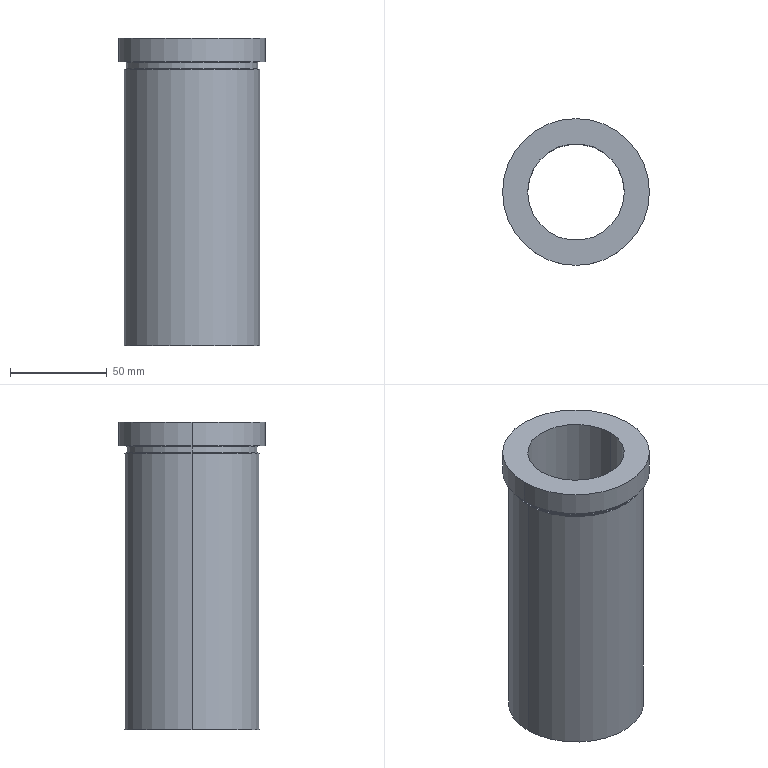Part | Creo | 1 solid | 24 faces | box 76 x 76 x 159 mm | volume 307086 mm3 | torus 12 | cylinder 8 | plane 4 | commonest cylinder face diameters 50 x2 68 x2 70 x2 76 x2
STEP:
#1=CARTESIAN_POINT('',(-237.,347.,144.5));
#2=VERTEX_POINT('',#1);
#3=CARTESIAN_POINT('',(-307.,347.,144.5));
#4=VERTEX_POINT('',#3);
#5=CARTESIAN_POINT('',(-272.,347.,144.5));
#6=DIRECTION('',(0.,0.,1.));
#7=DIRECTION('',(1.,0.,0.));
#8=AXIS2_PLACEMENT_3D('',#5,#6,#7);
#9=CIRCLE('',#8,35.);
#10=EDGE_CURVE('',#2,#4,#9,.T.);
#11=ORIENTED_EDGE('',*,*,#10,.T.);
#12=CARTESIAN_POINT('',(-307.,347.,1.5));
#13=VERTEX_POINT('',#12);
#14=CARTESIAN_POINT('',(-307.,347.,1.5));
#15=DIRECTION('',(0.,0.,1.));
#16=VECTOR('',#15,143.);
#17=LINE('',#14,#16);
#18=EDGE_CURVE('',#13,#4,#17,.T.);
#19=ORIENTED_EDGE('',*,*,#18,.F.);
#20=CARTESIAN_POINT('',(-237.,347.,1.5));
#21=VERTEX_POINT('',#20);
#22=CARTESIAN_POINT('',(-272.,347.,1.5));
#23=DIRECTION('',(0.,0.,-1.));
#24=DIRECTION('',(-1.,0.,0.));
#25=AXIS2_PLACEMENT_3D('',#22,#23,#24);
#26=CIRCLE('',#25,35.);
#27=EDGE_CURVE('',#13,#21,#26,.T.);
#28=ORIENTED_EDGE('',*,*,#27,.T.);
#29=CARTESIAN_POINT('',(-237.,347.,1.5));
#30=DIRECTION('',(0.,0.,1.));
#31=VECTOR('',#30,143.);
#32=LINE('',#29,#31);
#33=EDGE_CURVE('',#21,#2,#32,.T.);
#34=ORIENTED_EDGE('',*,*,#33,.T.);
#35=EDGE_LOOP('',(#11,#19,#28,#34));
#36=FACE_OUTER_BOUND('',#35,.F.);
#37=CARTESIAN_POINT('',(-272.,347.,1.5));
#38=DIRECTION('',(0.,0.,1.));
#39=DIRECTION('',(1.,0.,0.));
#40=AXIS2_PLACEMENT_3D('',#37,#38,#39);
#41=CYLINDRICAL_SURFACE('',#40,35.);
#42=ADVANCED_FACE('',(#36),#41,.T.);
#43=CARTESIAN_POINT('',(-272.,347.,144.5));
#44=DIRECTION('',(0.,0.,1.));
#45=DIRECTION('',(-1.,0.,0.));
#46=AXIS2_PLACEMENT_3D('',#43,#44,#45);
#47=CIRCLE('',#46,35.);
#48=EDGE_CURVE('',#4,#2,#47,.T.);
#49=ORIENTED_EDGE('',*,*,#48,.F.);
#50=ORIENTED_EDGE('',*,*,#10,.F.);
#51=EDGE_LOOP('',(#49,#50));
#52=FACE_OUTER_BOUND('',#51,.F.);
#53=CARTESIAN_POINT('',(-306.5,347.,144.5));
#54=VERTEX_POINT('',#53);
#55=CARTESIAN_POINT('',(-237.5,347.,144.5));
#56=VERTEX_POINT('',#55);
#57=CARTESIAN_POINT('',(-272.,347.,144.5));
#58=DIRECTION('',(0.,0.,-1.));
#59=DIRECTION('',(-1.,0.,0.));
#60=AXIS2_PLACEMENT_3D('',#57,#58,#59);
#61=CIRCLE('',#60,34.5);
#62=EDGE_CURVE('',#54,#56,#61,.T.);
#63=ORIENTED_EDGE('',*,*,#62,.F.);
#64=CARTESIAN_POINT('',(-272.,347.,144.5));
#65=DIRECTION('',(0.,0.,-1.));
#66=DIRECTION('',(1.,0.,0.));
#67=AXIS2_PLACEMENT_3D('',#64,#65,#66);
#68=CIRCLE('',#67,34.5);
#69=EDGE_CURVE('',#56,#54,#68,.T.);
#70=ORIENTED_EDGE('',*,*,#69,.F.);
#71=EDGE_LOOP('',(#63,#70));
#72=FACE_BOUND('',#71,.F.);
#73=CARTESIAN_POINT('',(-238.,347.,144.5));
#74=DIRECTION('',(0.,0.,-1.));
#75=DIRECTION('',(-1.,0.,0.));
#76=AXIS2_PLACEMENT_3D('',#73,#74,#75);
#77=PLANE('',#76);
#78=ADVANCED_FACE('',(#52,#72),#77,.F.);
#79=ORIENTED_EDGE('',*,*,#62,.T.);
#80=CARTESIAN_POINT('',(-237.854,347.,144.646));
#81=VERTEX_POINT('',#80);
#82=CARTESIAN_POINT('',(-237.5,347.,145.));
#83=DIRECTION('',(0.,1.,0.));
#84=DIRECTION('',(0.,0.,-1.));
#85=AXIS2_PLACEMENT_3D('',#82,#83,#84);
#86=CIRCLE('',#85,0.5);
#87=EDGE_CURVE('',#56,#81,#86,.T.);
#88=ORIENTED_EDGE('',*,*,#87,.T.);
#89=CARTESIAN_POINT('',(-306.146,347.,144.646));
#90=VERTEX_POINT('',#89);
#91=CARTESIAN_POINT('',(-272.,347.,144.646));
#92=DIRECTION('',(0.,0.,-1.));
#93=DIRECTION('',(-1.,0.,0.));
#94=AXIS2_PLACEMENT_3D('',#91,#92,#93);
#95=CIRCLE('',#94,34.146);
#96=EDGE_CURVE('',#90,#81,#95,.T.);
#97=ORIENTED_EDGE('',*,*,#96,.F.);
#98=CARTESIAN_POINT('',(-306.5,347.,145.));
#99=DIRECTION('',(0.,-1.,0.));
#100=DIRECTION('',(0.,0.,-1.));
#101=AXIS2_PLACEMENT_3D('',#98,#99,#100);
#102=CIRCLE('',#101,0.5);
#103=EDGE_CURVE('',#54,#90,#102,.T.);
#104=ORIENTED_EDGE('',*,*,#103,.F.);
#105=EDGE_LOOP('',(#79,#88,#97,#104));
#106=FACE_OUTER_BOUND('',#105,.F.);
#107=CARTESIAN_POINT('',(-272.,347.,145.));
#108=DIRECTION('',(0.,0.,-1.));
#109=DIRECTION('',(-1.,0.,0.));
#110=AXIS2_PLACEMENT_3D('',#107,#108,#109);
#111=TOROIDAL_SURFACE('',#110,34.5,0.5);
#112=ADVANCED_FACE('',(#106),#111,.F.);
#113=ORIENTED_EDGE('',*,*,#69,.T.);
#114=ORIENTED_EDGE('',*,*,#103,.T.);
#115=CARTESIAN_POINT('',(-272.,347.,144.646));
#116=DIRECTION('',(0.,0.,-1.));
#117=DIRECTION('',(1.,0.,0.));
#118=AXIS2_PLACEMENT_3D('',#115,#116,#117);
#119=CIRCLE('',#118,34.146);
#120=EDGE_CURVE('',#81,#90,#119,.T.);
#121=ORIENTED_EDGE('',*,*,#120,.F.);
#122=ORIENTED_EDGE('',*,*,#87,.F.);
#123=EDGE_LOOP('',(#113,#114,#121,#122));
#124=FACE_OUTER_BOUND('',#123,.F.);
#125=CARTESIAN_POINT('',(-272.,347.,145.));
#126=DIRECTION('',(0.,0.,-1.));
#127=DIRECTION('',(-1.,0.,0.));
#128=AXIS2_PLACEMENT_3D('',#125,#126,#127);
#129=TOROIDAL_SURFACE('',#128,34.5,0.5);
#130=ADVANCED_FACE('',(#124),#129,.F.);
#131=CARTESIAN_POINT('',(-238.,347.,145.));
#132=VERTEX_POINT('',#131);
#133=CARTESIAN_POINT('',(-306.,347.,145.));
#134=VERTEX_POINT('',#133);
#135=CARTESIAN_POINT('',(-272.,347.,145.));
#136=DIRECTION('',(0.,0.,-1.));
#137=DIRECTION('',(1.,0.,0.));
#138=AXIS2_PLACEMENT_3D('',#135,#136,#137);
#139=CIRCLE('',#138,34.);
#140=EDGE_CURVE('',#132,#134,#139,.T.);
#141=ORIENTED_EDGE('',*,*,#140,.F.);
#142=CARTESIAN_POINT('',(-237.5,347.,145.));
#143=DIRECTION('',(0.,1.,0.));
#144=DIRECTION('',(-0.7071,0.,-0.7071));
#145=AXIS2_PLACEMENT_3D('',#142,#143,#144);
#146=CIRCLE('',#145,0.5);
#147=EDGE_CURVE('',#81,#132,#146,.T.);
#148=ORIENTED_EDGE('',*,*,#147,.F.);
#149=ORIENTED_EDGE('',*,*,#120,.T.);
#150=CARTESIAN_POINT('',(-306.5,347.,145.));
#151=DIRECTION('',(0.,-1.,0.));
#152=DIRECTION('',(0.7071,0.,-0.7071));
#153=AXIS2_PLACEMENT_3D('',#150,#151,#152);
#154=CIRCLE('',#153,0.5);
#155=EDGE_CURVE('',#90,#134,#154,.T.);
#156=ORIENTED_EDGE('',*,*,#155,.T.);
#157=EDGE_LOOP('',(#141,#148,#149,#156));
#158=FACE_OUTER_BOUND('',#157,.F.);
#159=CARTESIAN_POINT('',(-272.,347.,145.));
#160=DIRECTION('',(0.,0.,-1.));
#161=DIRECTION('',(-1.,0.,0.));
#162=AXIS2_PLACEMENT_3D('',#159,#160,#161);
#163=TOROIDAL_SURFACE('',#162,34.5,0.5);
#164=ADVANCED_FACE('',(#158),#163,.F.);
#165=ORIENTED_EDGE('',*,*,#140,.T.);
#166=CARTESIAN_POINT('',(-306.,347.,148.));
#167=VERTEX_POINT('',#166);
#168=CARTESIAN_POINT('',(-306.,347.,148.));
#169=DIRECTION('',(0.,0.,-1.));
#170=VECTOR('',#169,3.);
#171=LINE('',#168,#170);
#172=EDGE_CURVE('',#167,#134,#171,.T.);
#173=ORIENTED_EDGE('',*,*,#172,.F.);
#174=CARTESIAN_POINT('',(-238.,347.,148.));
#175=VERTEX_POINT('',#174);
#176=CARTESIAN_POINT('',(-272.,347.,148.));
#177=DIRECTION('',(0.,0.,1.));
#178=DIRECTION('',(-1.,0.,0.));
#179=AXIS2_PLACEMENT_3D('',#176,#177,#178);
#180=CIRCLE('',#179,34.);
#181=EDGE_CURVE('',#167,#175,#180,.T.);
#182=ORIENTED_EDGE('',*,*,#181,.T.);
#183=CARTESIAN_POINT('',(-238.,347.,148.));
#184=DIRECTION('',(0.,0.,-1.));
#185=VECTOR('',#184,3.);
#186=LINE('',#183,#185);
#187=EDGE_CURVE('',#175,#132,#186,.T.);
#188=ORIENTED_EDGE('',*,*,#187,.T.);
#189=EDGE_LOOP('',(#165,#173,#182,#188));
#190=FACE_OUTER_BOUND('',#189,.F.);
#191=CARTESIAN_POINT('',(-272.,347.,100.707));
#192=DIRECTION('',(0.,0.,-1.));
#193=DIRECTION('',(-1.,0.,0.));
#194=AXIS2_PLACEMENT_3D('',#191,#192,#193);
#195=CYLINDRICAL_SURFACE('',#194,34.);
#196=ADVANCED_FACE('',(#190),#195,.T.);
#197=CARTESIAN_POINT('',(-272.,347.,145.));
#198=DIRECTION('',(0.,0.,-1.));
#199=DIRECTION('',(-1.,0.,0.));
#200=AXIS2_PLACEMENT_3D('',#197,#198,#199);
#201=CIRCLE('',#200,34.);
#202=EDGE_CURVE('',#134,#132,#201,.T.);
#203=ORIENTED_EDGE('',*,*,#202,.T.);
#204=ORIENTED_EDGE('',*,*,#187,.F.);
#205=CARTESIAN_POINT('',(-272.,347.,148.));
#206=DIRECTION('',(0.,0.,1.));
#207=DIRECTION('',(1.,0.,0.));
#208=AXIS2_PLACEMENT_3D('',#205,#206,#207);
#209=CIRCLE('',#208,34.);
#210=EDGE_CURVE('',#175,#167,#209,.T.);
#211=ORIENTED_EDGE('',*,*,#210,.T.);
#212=ORIENTED_EDGE('',*,*,#172,.T.);
#213=EDGE_LOOP('',(#203,#204,#211,#212));
#214=FACE_OUTER_BOUND('',#213,.F.);
#215=CARTESIAN_POINT('',(-272.,347.,100.707));
#216=DIRECTION('',(0.,0.,-1.));
#217=DIRECTION('',(-1.,0.,0.));
#218=AXIS2_PLACEMENT_3D('',#215,#216,#217);
#219=CYLINDRICAL_SURFACE('',#218,34.);
#220=ADVANCED_FACE('',(#214),#219,.T.);
#221=ORIENTED_EDGE('',*,*,#202,.F.);
#222=ORIENTED_EDGE('',*,*,#155,.F.);
#223=ORIENTED_EDGE('',*,*,#96,.T.);
#224=ORIENTED_EDGE('',*,*,#147,.T.);
#225=EDGE_LOOP('',(#221,#222,#223,#224));
#226=FACE_OUTER_BOUND('',#225,.F.);
#227=CARTESIAN_POINT('',(-272.,347.,145.));
#228=DIRECTION('',(0.,0.,-1.));
#229=DIRECTION('',(-1.,0.,0.));
#230=AXIS2_PLACEMENT_3D('',#227,#228,#229);
#231=TOROIDAL_SURFACE('',#230,34.5,0.5);
#232=ADVANCED_FACE('',(#226),#231,.F.);
#233=ORIENTED_EDGE('',*,*,#210,.F.);
#234=CARTESIAN_POINT('',(-237.854,347.,148.354));
#235=VERTEX_POINT('',#234);
#236=CARTESIAN_POINT('',(-237.5,347.,148.));
#237=DIRECTION('',(0.,-1.,0.));
#238=DIRECTION('',(-0.7071,0.,0.7071));
#239=AXIS2_PLACEMENT_3D('',#236,#237,#238);
#240=CIRCLE('',#239,0.5);
#241=EDGE_CURVE('',#235,#175,#240,.T.);
#242=ORIENTED_EDGE('',*,*,#241,.F.);
#243=CARTESIAN_POINT('',(-306.146,347.,148.354));
#244=VERTEX_POINT('',#243);
#245=CARTESIAN_POINT('',(-272.,347.,148.354));
#246=DIRECTION('',(0.,0.,1.));
#247=DIRECTION('',(1.,0.,0.));
#248=AXIS2_PLACEMENT_3D('',#245,#246,#247);
#249=CIRCLE('',#248,34.146);
#250=EDGE_CURVE('',#235,#244,#249,.T.);
#251=ORIENTED_EDGE('',*,*,#250,.T.);
#252=CARTESIAN_POINT('',(-306.5,347.,148.));
#253=DIRECTION('',(0.,1.,0.));
#254=DIRECTION('',(0.7071,0.,0.7071));
#255=AXIS2_PLACEMENT_3D('',#252,#253,#254);
#256=CIRCLE('',#255,0.5);
#257=EDGE_CURVE('',#244,#167,#256,.T.);
#258=ORIENTED_EDGE('',*,*,#257,.T.);
#259=EDGE_LOOP('',(#233,#242,#251,#258));
#260=FACE_OUTER_BOUND('',#259,.F.);
#261=CARTESIAN_POINT('',(-272.,347.,148.));
#262=DIRECTION('',(0.,0.,1.));
#263=DIRECTION('',(1.,0.,0.));
#264=AXIS2_PLACEMENT_3D('',#261,#262,#263);
#265=TOROIDAL_SURFACE('',#264,34.5,0.5);
#266=ADVANCED_FACE('',(#260),#265,.F.);
#267=ORIENTED_EDGE('',*,*,#181,.F.);
#268=ORIENTED_EDGE('',*,*,#257,.F.);
#269=CARTESIAN_POINT('',(-272.,347.,148.354));
#270=DIRECTION('',(0.,0.,1.));
#271=DIRECTION('',(-1.,0.,0.));
#272=AXIS2_PLACEMENT_3D('',#269,#270,#271);
#273=CIRCLE('',#272,34.146);
#274=EDGE_CURVE('',#244,#235,#273,.T.);
#275=ORIENTED_EDGE('',*,*,#274,.T.);
#276=ORIENTED_EDGE('',*,*,#241,.T.);
#277=EDGE_LOOP('',(#267,#268,#275,#276));
#278=FACE_OUTER_BOUND('',#277,.F.);
#279=CARTESIAN_POINT('',(-272.,347.,148.));
#280=DIRECTION('',(0.,0.,1.));
#281=DIRECTION('',(1.,0.,0.));
#282=AXIS2_PLACEMENT_3D('',#279,#280,#281);
#283=TOROIDAL_SURFACE('',#282,34.5,0.5);
#284=ADVANCED_FACE('',(#278),#283,.F.);
#285=CARTESIAN_POINT('',(-306.5,347.,148.5));
#286=VERTEX_POINT('',#285);
#287=CARTESIAN_POINT('',(-237.5,347.,148.5));
#288=VERTEX_POINT('',#287);
#289=CARTESIAN_POINT('',(-272.,347.,148.5));
#290=DIRECTION('',(0.,0.,1.));
#291=DIRECTION('',(-1.,0.,0.));
#292=AXIS2_PLACEMENT_3D('',#289,#290,#291);
#293=CIRCLE('',#292,34.5);
#294=EDGE_CURVE('',#286,#288,#293,.T.);
#295=ORIENTED_EDGE('',*,*,#294,.T.);
#296=CARTESIAN_POINT('',(-237.5,347.,148.));
#297=DIRECTION('',(0.,-1.,0.));
#298=DIRECTION('',(0.,0.,1.));
#299=AXIS2_PLACEMENT_3D('',#296,#297,#298);
#300=CIRCLE('',#299,0.5);
#301=EDGE_CURVE('',#288,#235,#300,.T.);
#302=ORIENTED_EDGE('',*,*,#301,.T.);
#303=ORIENTED_EDGE('',*,*,#274,.F.);
#304=CARTESIAN_POINT('',(-306.5,347.,148.));
#305=DIRECTION('',(0.,1.,0.));
#306=DIRECTION('',(0.,0.,1.));
#307=AXIS2_PLACEMENT_3D('',#304,#305,#306);
#308=CIRCLE('',#307,0.5);
#309=EDGE_CURVE('',#286,#244,#308,.T.);
#310=ORIENTED_EDGE('',*,*,#309,.F.);
#311=EDGE_LOOP('',(#295,#302,#303,#310));
#312=FACE_OUTER_BOUND('',#311,.F.);
#313=CARTESIAN_POINT('',(-272.,347.,148.));
#314=DIRECTION('',(0.,0.,1.));
#315=DIRECTION('',(1.,0.,0.));
#316=AXIS2_PLACEMENT_3D('',#313,#314,#315);
#317=TOROIDAL_SURFACE('',#316,34.5,0.5);
#318=ADVANCED_FACE('',(#312),#317,.F.);
#319=CARTESIAN_POINT('',(-234.,347.,148.5));
#320=VERTEX_POINT('',#319);
#321=CARTESIAN_POINT('',(-310.,347.,148.5));
#322=VERTEX_POINT('',#321);
#323=CARTESIAN_POINT('',(-272.,347.,148.5));
#324=DIRECTION('',(0.,0.,-1.));
#325=DIRECTION('',(1.,0.,0.));
#326=AXIS2_PLACEMENT_3D('',#323,#324,#325);
#327=CIRCLE('',#326,38.);
#328=EDGE_CURVE('',#320,#322,#327,.T.);
#329=ORIENTED_EDGE('',*,*,#328,.F.);
#330=CARTESIAN_POINT('',(-272.,347.,148.5));
#331=DIRECTION('',(0.,0.,-1.));
#332=DIRECTION('',(-1.,0.,0.));
#333=AXIS2_PLACEMENT_3D('',#330,#331,#332);
#334=CIRCLE('',#333,38.);
#335=EDGE_CURVE('',#322,#320,#334,.T.);
#336=ORIENTED_EDGE('',*,*,#335,.F.);
#337=EDGE_LOOP('',(#329,#336));
#338=FACE_OUTER_BOUND('',#337,.F.);
#339=CARTESIAN_POINT('',(-272.,347.,148.5));
#340=DIRECTION('',(0.,0.,1.));
#341=DIRECTION('',(1.,0.,0.));
#342=AXIS2_PLACEMENT_3D('',#339,#340,#341);
#343=CIRCLE('',#342,34.5);
#344=EDGE_CURVE('',#288,#286,#343,.T.);
#345=ORIENTED_EDGE('',*,*,#344,.F.);
#346=ORIENTED_EDGE('',*,*,#294,.F.);
#347=EDGE_LOOP('',(#345,#346));
#348=FACE_BOUND('',#347,.F.);
#349=CARTESIAN_POINT('',(-272.,347.,148.5));
#350=DIRECTION('',(0.,0.,1.));
#351=DIRECTION('',(1.,0.,0.));
#352=AXIS2_PLACEMENT_3D('',#349,#350,#351);
#353=PLANE('',#352);
#354=ADVANCED_FACE('',(#338,#348),#353,.F.);
#355=ORIENTED_EDGE('',*,*,#344,.T.);
#356=ORIENTED_EDGE('',*,*,#309,.T.);
#357=ORIENTED_EDGE('',*,*,#250,.F.);
#358=ORIENTED_EDGE('',*,*,#301,.F.);
#359=EDGE_LOOP('',(#355,#356,#357,#358));
#360=FACE_OUTER_BOUND('',#359,.F.);
#361=CARTESIAN_POINT('',(-272.,347.,148.));
#362=DIRECTION('',(0.,0.,1.));
#363=DIRECTION('',(1.,0.,0.));
#364=AXIS2_PLACEMENT_3D('',#361,#362,#363);
#365=TOROIDAL_SURFACE('',#364,34.5,0.5);
#366=ADVANCED_FACE('',(#360),#365,.F.);
#367=ORIENTED_EDGE('',*,*,#328,.T.);
#368=CARTESIAN_POINT('',(-310.,347.,160.5));
#369=VERTEX_POINT('',#368);
#370=CARTESIAN_POINT('',(-310.,347.,148.5));
#371=DIRECTION('',(0.,0.,1.));
#372=VECTOR('',#371,12.);
#373=LINE('',#370,#372);
#374=EDGE_CURVE('',#322,#369,#373,.T.);
#375=ORIENTED_EDGE('',*,*,#374,.T.);
#376=CARTESIAN_POINT('',(-234.,347.,160.5));
#377=VERTEX_POINT('',#376);
#378=CARTESIAN_POINT('',(-272.,347.,160.5));
#379=DIRECTION('',(0.,0.,1.));
#380=DIRECTION('',(-1.,0.,0.));
#381=AXIS2_PLACEMENT_3D('',#378,#379,#380);
#382=CIRCLE('',#381,38.);
#383=EDGE_CURVE('',#369,#377,#382,.T.);
#384=ORIENTED_EDGE('',*,*,#383,.T.);
#385=CARTESIAN_POINT('',(-234.,347.,148.5));
#386=DIRECTION('',(0.,0.,1.));
#387=VECTOR('',#386,12.);
#388=LINE('',#385,#387);
#389=EDGE_CURVE('',#320,#377,#388,.T.);
#390=ORIENTED_EDGE('',*,*,#389,.F.);
#391=EDGE_LOOP('',(#367,#375,#384,#390));
#392=FACE_OUTER_BOUND('',#391,.F.);
#393=CARTESIAN_POINT('',(-272.,347.,148.5));
#394=DIRECTION('',(0.,0.,1.));
#395=DIRECTION('',(1.,0.,0.));
#396=AXIS2_PLACEMENT_3D('',#393,#394,#395);
#397=CYLINDRICAL_SURFACE('',#396,38.);
#398=ADVANCED_FACE('',(#392),#397,.T.);
#399=ORIENTED_EDGE('',*,*,#335,.T.);
#400=ORIENTED_EDGE('',*,*,#389,.T.);
#401=CARTESIAN_POINT('',(-272.,347.,160.5));
#402=DIRECTION('',(0.,0.,1.));
#403=DIRECTION('',(1.,0.,0.));
#404=AXIS2_PLACEMENT_3D('',#401,#402,#403);
#405=CIRCLE('',#404,38.);
#406=EDGE_CURVE('',#377,#369,#405,.T.);
#407=ORIENTED_EDGE('',*,*,#406,.T.);
#408=ORIENTED_EDGE('',*,*,#374,.F.);
#409=EDGE_LOOP('',(#399,#400,#407,#408));
#410=FACE_OUTER_BOUND('',#409,.F.);
#411=CARTESIAN_POINT('',(-272.,347.,148.5));
#412=DIRECTION('',(0.,0.,1.));
#413=DIRECTION('',(1.,0.,0.));
#414=AXIS2_PLACEMENT_3D('',#411,#412,#413);
#415=CYLINDRICAL_SURFACE('',#414,38.);
#416=ADVANCED_FACE('',(#410),#415,.T.);
#417=ORIENTED_EDGE('',*,*,#406,.F.);
#418=ORIENTED_EDGE('',*,*,#383,.F.);
#419=EDGE_LOOP('',(#417,#418));
#420=FACE_OUTER_BOUND('',#419,.F.);
#421=CARTESIAN_POINT('',(-247.,347.,160.5));
#422=VERTEX_POINT('',#421);
#423=CARTESIAN_POINT('',(-297.,347.,160.5));
#424=VERTEX_POINT('',#423);
#425=CARTESIAN_POINT('',(-272.,347.,160.5));
#426=DIRECTION('',(0.,0.,-1.));
#427=DIRECTION('',(1.,0.,0.));
#428=AXIS2_PLACEMENT_3D('',#425,#426,#427);
#429=CIRCLE('',#428,25.);
#430=EDGE_CURVE('',#422,#424,#429,.T.);
#431=ORIENTED_EDGE('',*,*,#430,.F.);
#432=CARTESIAN_POINT('',(-272.,347.,160.5));
#433=DIRECTION('',(0.,0.,-1.));
#434=DIRECTION('',(-1.,0.,0.));
#435=AXIS2_PLACEMENT_3D('',#432,#433,#434);
#436=CIRCLE('',#435,25.);
#437=EDGE_CURVE('',#424,#422,#436,.T.);
#438=ORIENTED_EDGE('',*,*,#437,.F.);
#439=EDGE_LOOP('',(#431,#438));
#440=FACE_BOUND('',#439,.F.);
#441=CARTESIAN_POINT('',(-272.,347.,160.5));
#442=DIRECTION('',(0.,0.,1.));
#443=DIRECTION('',(1.,0.,0.));
#444=AXIS2_PLACEMENT_3D('',#441,#442,#443);
#445=PLANE('',#444);
#446=ADVANCED_FACE('',(#420,#440),#445,.T.);
#447=CARTESIAN_POINT('',(-297.,347.,2.5));
#448=VERTEX_POINT('',#447);
#449=CARTESIAN_POINT('',(-247.,347.,2.5));
#450=VERTEX_POINT('',#449);
#451=CARTESIAN_POINT('',(-272.,347.,2.5));
#452=DIRECTION('',(0.,0.,1.));
#453=DIRECTION('',(-1.,0.,0.));
#454=AXIS2_PLACEMENT_3D('',#451,#452,#453);
#455=CIRCLE('',#454,25.);
#456=EDGE_CURVE('',#448,#450,#455,.T.);
#457=ORIENTED_EDGE('',*,*,#456,.T.);
#458=CARTESIAN_POINT('',(-247.,347.,2.5));
#459=DIRECTION('',(0.,0.,1.));
#460=VECTOR('',#459,158.);
#461=LINE('',#458,#460);
#462=EDGE_CURVE('',#450,#422,#461,.T.);
#463=ORIENTED_EDGE('',*,*,#462,.T.);
#464=ORIENTED_EDGE('',*,*,#430,.T.);
#465=CARTESIAN_POINT('',(-297.,347.,2.5));
#466=DIRECTION('',(0.,0.,1.));
#467=VECTOR('',#466,158.);
#468=LINE('',#465,#467);
#469=EDGE_CURVE('',#448,#424,#468,.T.);
#470=ORIENTED_EDGE('',*,*,#469,.F.);
#471=EDGE_LOOP('',(#457,#463,#464,#470));
#472=FACE_OUTER_BOUND('',#471,.F.);
#473=CARTESIAN_POINT('',(-272.,347.,1.5));
#474=DIRECTION('',(0.,0.,1.));
#475=DIRECTION('',(1.,0.,0.));
#476=AXIS2_PLACEMENT_3D('',#473,#474,#475);
#477=CYLINDRICAL_SURFACE('',#476,25.);
#478=ADVANCED_FACE('',(#472),#477,.F.);
#479=ORIENTED_EDGE('',*,*,#456,.F.);
#480=CARTESIAN_POINT('',(-297.293,347.,1.793));
#481=VERTEX_POINT('',#480);
#482=CARTESIAN_POINT('',(-298.,347.,2.5));
#483=DIRECTION('',(0.,1.,0.));
#484=DIRECTION('',(1.,0.,0.));
#485=AXIS2_PLACEMENT_3D('',#482,#483,#484);
#486=CIRCLE('',#485,1.);
#487=EDGE_CURVE('',#448,#481,#486,.T.);
#488=ORIENTED_EDGE('',*,*,#487,.T.);
#489=CARTESIAN_POINT('',(-246.707,347.,1.793));
#490=VERTEX_POINT('',#489);
#491=CARTESIAN_POINT('',(-272.,347.,1.793));
#492=DIRECTION('',(0.,0.,1.));
#493=DIRECTION('',(-1.,0.,0.));
#494=AXIS2_PLACEMENT_3D('',#491,#492,#493);
#495=CIRCLE('',#494,25.293);
#496=EDGE_CURVE('',#481,#490,#495,.T.);
#497=ORIENTED_EDGE('',*,*,#496,.T.);
#498=CARTESIAN_POINT('',(-246.,347.,2.5));
#499=DIRECTION('',(0.,-1.,0.));
#500=DIRECTION('',(-1.,0.,0.));
#501=AXIS2_PLACEMENT_3D('',#498,#499,#500);
#502=CIRCLE('',#501,1.);
#503=EDGE_CURVE('',#450,#490,#502,.T.);
#504=ORIENTED_EDGE('',*,*,#503,.F.);
#505=EDGE_LOOP('',(#479,#488,#497,#504));
#506=FACE_OUTER_BOUND('',#505,.F.);
#507=CARTESIAN_POINT('',(-272.,347.,2.5));
#508=DIRECTION('',(0.,0.,1.));
#509=DIRECTION('',(1.,0.,0.));
#510=AXIS2_PLACEMENT_3D('',#507,#508,#509);
#511=TOROIDAL_SURFACE('',#510,26.,1.);
#512=ADVANCED_FACE('',(#506),#511,.T.);
#513=CARTESIAN_POINT('',(-272.,347.,2.5));
#514=DIRECTION('',(0.,0.,1.));
#515=DIRECTION('',(1.,0.,0.));
#516=AXIS2_PLACEMENT_3D('',#513,#514,#515);
#517=CIRCLE('',#516,25.);
#518=EDGE_CURVE('',#450,#448,#517,.T.);
#519=ORIENTED_EDGE('',*,*,#518,.F.);
#520=ORIENTED_EDGE('',*,*,#503,.T.);
#521=CARTESIAN_POINT('',(-272.,347.,1.793));
#522=DIRECTION('',(0.,0.,1.));
#523=DIRECTION('',(1.,0.,0.));
#524=AXIS2_PLACEMENT_3D('',#521,#522,#523);
#525=CIRCLE('',#524,25.293);
#526=EDGE_CURVE('',#490,#481,#525,.T.);
#527=ORIENTED_EDGE('',*,*,#526,.T.);
#528=ORIENTED_EDGE('',*,*,#487,.F.);
#529=EDGE_LOOP('',(#519,#520,#527,#528));
#530=FACE_OUTER_BOUND('',#529,.F.);
#531=CARTESIAN_POINT('',(-272.,347.,2.5));
#532=DIRECTION('',(0.,0.,1.));
#533=DIRECTION('',(1.,0.,0.));
#534=AXIS2_PLACEMENT_3D('',#531,#532,#533);
#535=TOROIDAL_SURFACE('',#534,26.,1.);
#536=ADVANCED_FACE('',(#530),#535,.T.);
#537=ORIENTED_EDGE('',*,*,#518,.T.);
#538=ORIENTED_EDGE('',*,*,#469,.T.);
#539=ORIENTED_EDGE('',*,*,#437,.T.);
#540=ORIENTED_EDGE('',*,*,#462,.F.);
#541=EDGE_LOOP('',(#537,#538,#539,#540));
#542=FACE_OUTER_BOUND('',#541,.F.);
#543=CARTESIAN_POINT('',(-272.,347.,1.5));
#544=DIRECTION('',(0.,0.,1.));
#545=DIRECTION('',(1.,0.,0.));
#546=AXIS2_PLACEMENT_3D('',#543,#544,#545);
#547=CYLINDRICAL_SURFACE('',#546,25.);
#548=ADVANCED_FACE('',(#542),#547,.F.);
#549=CARTESIAN_POINT('',(-246.,347.,1.5));
#550=VERTEX_POINT('',#549);
#551=CARTESIAN_POINT('',(-298.,347.,1.5));
#552=VERTEX_POINT('',#551);
#553=CARTESIAN_POINT('',(-272.,347.,1.5));
#554=DIRECTION('',(0.,0.,1.));
#555=DIRECTION('',(1.,0.,0.));
#556=AXIS2_PLACEMENT_3D('',#553,#554,#555);
#557=CIRCLE('',#556,26.);
#558=EDGE_CURVE('',#550,#552,#557,.T.);
#559=ORIENTED_EDGE('',*,*,#558,.T.);
#560=CARTESIAN_POINT('',(-298.,347.,2.5));
#561=DIRECTION('',(0.,1.,0.));
#562=DIRECTION('',(0.7071,0.,-0.7071));
#563=AXIS2_PLACEMENT_3D('',#560,#561,#562);
#564=CIRCLE('',#563,1.);
#565=EDGE_CURVE('',#481,#552,#564,.T.);
#566=ORIENTED_EDGE('',*,*,#565,.F.);
#567=ORIENTED_EDGE('',*,*,#526,.F.);
#568=CARTESIAN_POINT('',(-246.,347.,2.5));
#569=DIRECTION('',(0.,-1.,0.));
#570=DIRECTION('',(-0.7071,0.,-0.7071));
#571=AXIS2_PLACEMENT_3D('',#568,#569,#570);
#572=CIRCLE('',#571,1.);
#573=EDGE_CURVE('',#490,#550,#572,.T.);
#574=ORIENTED_EDGE('',*,*,#573,.T.);
#575=EDGE_LOOP('',(#559,#566,#567,#574));
#576=FACE_OUTER_BOUND('',#575,.F.);
#577=CARTESIAN_POINT('',(-272.,347.,2.5));
#578=DIRECTION('',(0.,0.,1.));
#579=DIRECTION('',(1.,0.,0.));
#580=AXIS2_PLACEMENT_3D('',#577,#578,#579);
#581=TOROIDAL_SURFACE('',#580,26.,1.);
#582=ADVANCED_FACE('',(#576),#581,.T.);
#583=CARTESIAN_POINT('',(-272.,347.,1.5));
#584=DIRECTION('',(0.,0.,-1.));
#585=DIRECTION('',(1.,0.,0.));
#586=AXIS2_PLACEMENT_3D('',#583,#584,#585);
#587=CIRCLE('',#586,35.);
#588=EDGE_CURVE('',#21,#13,#587,.T.);
#589=ORIENTED_EDGE('',*,*,#588,.F.);
#590=ORIENTED_EDGE('',*,*,#27,.F.);
#591=EDGE_LOOP('',(#589,#590));
#592=FACE_OUTER_BOUND('',#591,.F.);
#593=ORIENTED_EDGE('',*,*,#558,.F.);
#594=CARTESIAN_POINT('',(-272.,347.,1.5));
#595=DIRECTION('',(0.,0.,1.));
#596=DIRECTION('',(-1.,0.,0.));
#597=AXIS2_PLACEMENT_3D('',#594,#595,#596);
#598=CIRCLE('',#597,26.);
#599=EDGE_CURVE('',#552,#550,#598,.T.);
#600=ORIENTED_EDGE('',*,*,#599,.F.);
#601=EDGE_LOOP('',(#593,#600));
#602=FACE_BOUND('',#601,.F.);
#603=CARTESIAN_POINT('',(-272.,347.,1.5));
#604=DIRECTION('',(0.,0.,1.));
#605=DIRECTION('',(1.,0.,0.));
#606=AXIS2_PLACEMENT_3D('',#603,#604,#605);
#607=PLANE('',#606);
#608=ADVANCED_FACE('',(#592,#602),#607,.F.);
#609=ORIENTED_EDGE('',*,*,#599,.T.);
#610=ORIENTED_EDGE('',*,*,#573,.F.);
#611=ORIENTED_EDGE('',*,*,#496,.F.);
#612=ORIENTED_EDGE('',*,*,#565,.T.);
#613=EDGE_LOOP('',(#609,#610,#611,#612));
#614=FACE_OUTER_BOUND('',#613,.F.);
#615=CARTESIAN_POINT('',(-272.,347.,2.5));
#616=DIRECTION('',(0.,0.,1.));
#617=DIRECTION('',(1.,0.,0.));
#618=AXIS2_PLACEMENT_3D('',#615,#616,#617);
#619=TOROIDAL_SURFACE('',#618,26.,1.);
#620=ADVANCED_FACE('',(#614),#619,.T.);
#621=ORIENTED_EDGE('',*,*,#48,.T.);
#622=ORIENTED_EDGE('',*,*,#33,.F.);
#623=ORIENTED_EDGE('',*,*,#588,.T.);
#624=ORIENTED_EDGE('',*,*,#18,.T.);
#625=EDGE_LOOP('',(#621,#622,#623,#624));
#626=FACE_OUTER_BOUND('',#625,.F.);
#627=CARTESIAN_POINT('',(-272.,347.,1.5));
#628=DIRECTION('',(0.,0.,1.));
#629=DIRECTION('',(1.,0.,0.));
#630=AXIS2_PLACEMENT_3D('',#627,#628,#629);
#631=CYLINDRICAL_SURFACE('',#630,35.);
#632=ADVANCED_FACE('',(#626),#631,.T.);
#633=CLOSED_SHELL('',(#42,#78,#112,#130,#164,#196,#220,#232,#266,#284,#318,#354,#366,#398,#416,#446,#478,#512,#536,#548,#582,#608,#620,#632));
#634=MANIFOLD_SOLID_BREP('',#633);
#635=(LENGTH_UNIT()NAMED_UNIT(*)SI_UNIT(.MILLI.,.METRE.));
#636=UNCERTAINTY_MEASURE_WITH_UNIT(LENGTH_MEASURE(0.01919),#635,'','');
#637=(NAMED_UNIT(*)PLANE_ANGLE_UNIT()SI_UNIT($,.RADIAN.));
#638=PLANE_ANGLE_MEASURE_WITH_UNIT(PLANE_ANGLE_MEASURE(0.01745),#637);
#639=(CONVERSION_BASED_UNIT('DEGREE',#638)NAMED_UNIT(*)PLANE_ANGLE_UNIT());
#640=(NAMED_UNIT(*)SI_UNIT($,.STERADIAN.)SOLID_ANGLE_UNIT());
#641=(GEOMETRIC_REPRESENTATION_CONTEXT(3)GLOBAL_UNCERTAINTY_ASSIGNED_CONTEXT((#636))GLOBAL_UNIT_ASSIGNED_CONTEXT((#635,#639,#640))REPRESENTATION_CONTEXT('',''));
#642=ADVANCED_BREP_SHAPE_REPRESENTATION('',(#634),#641);